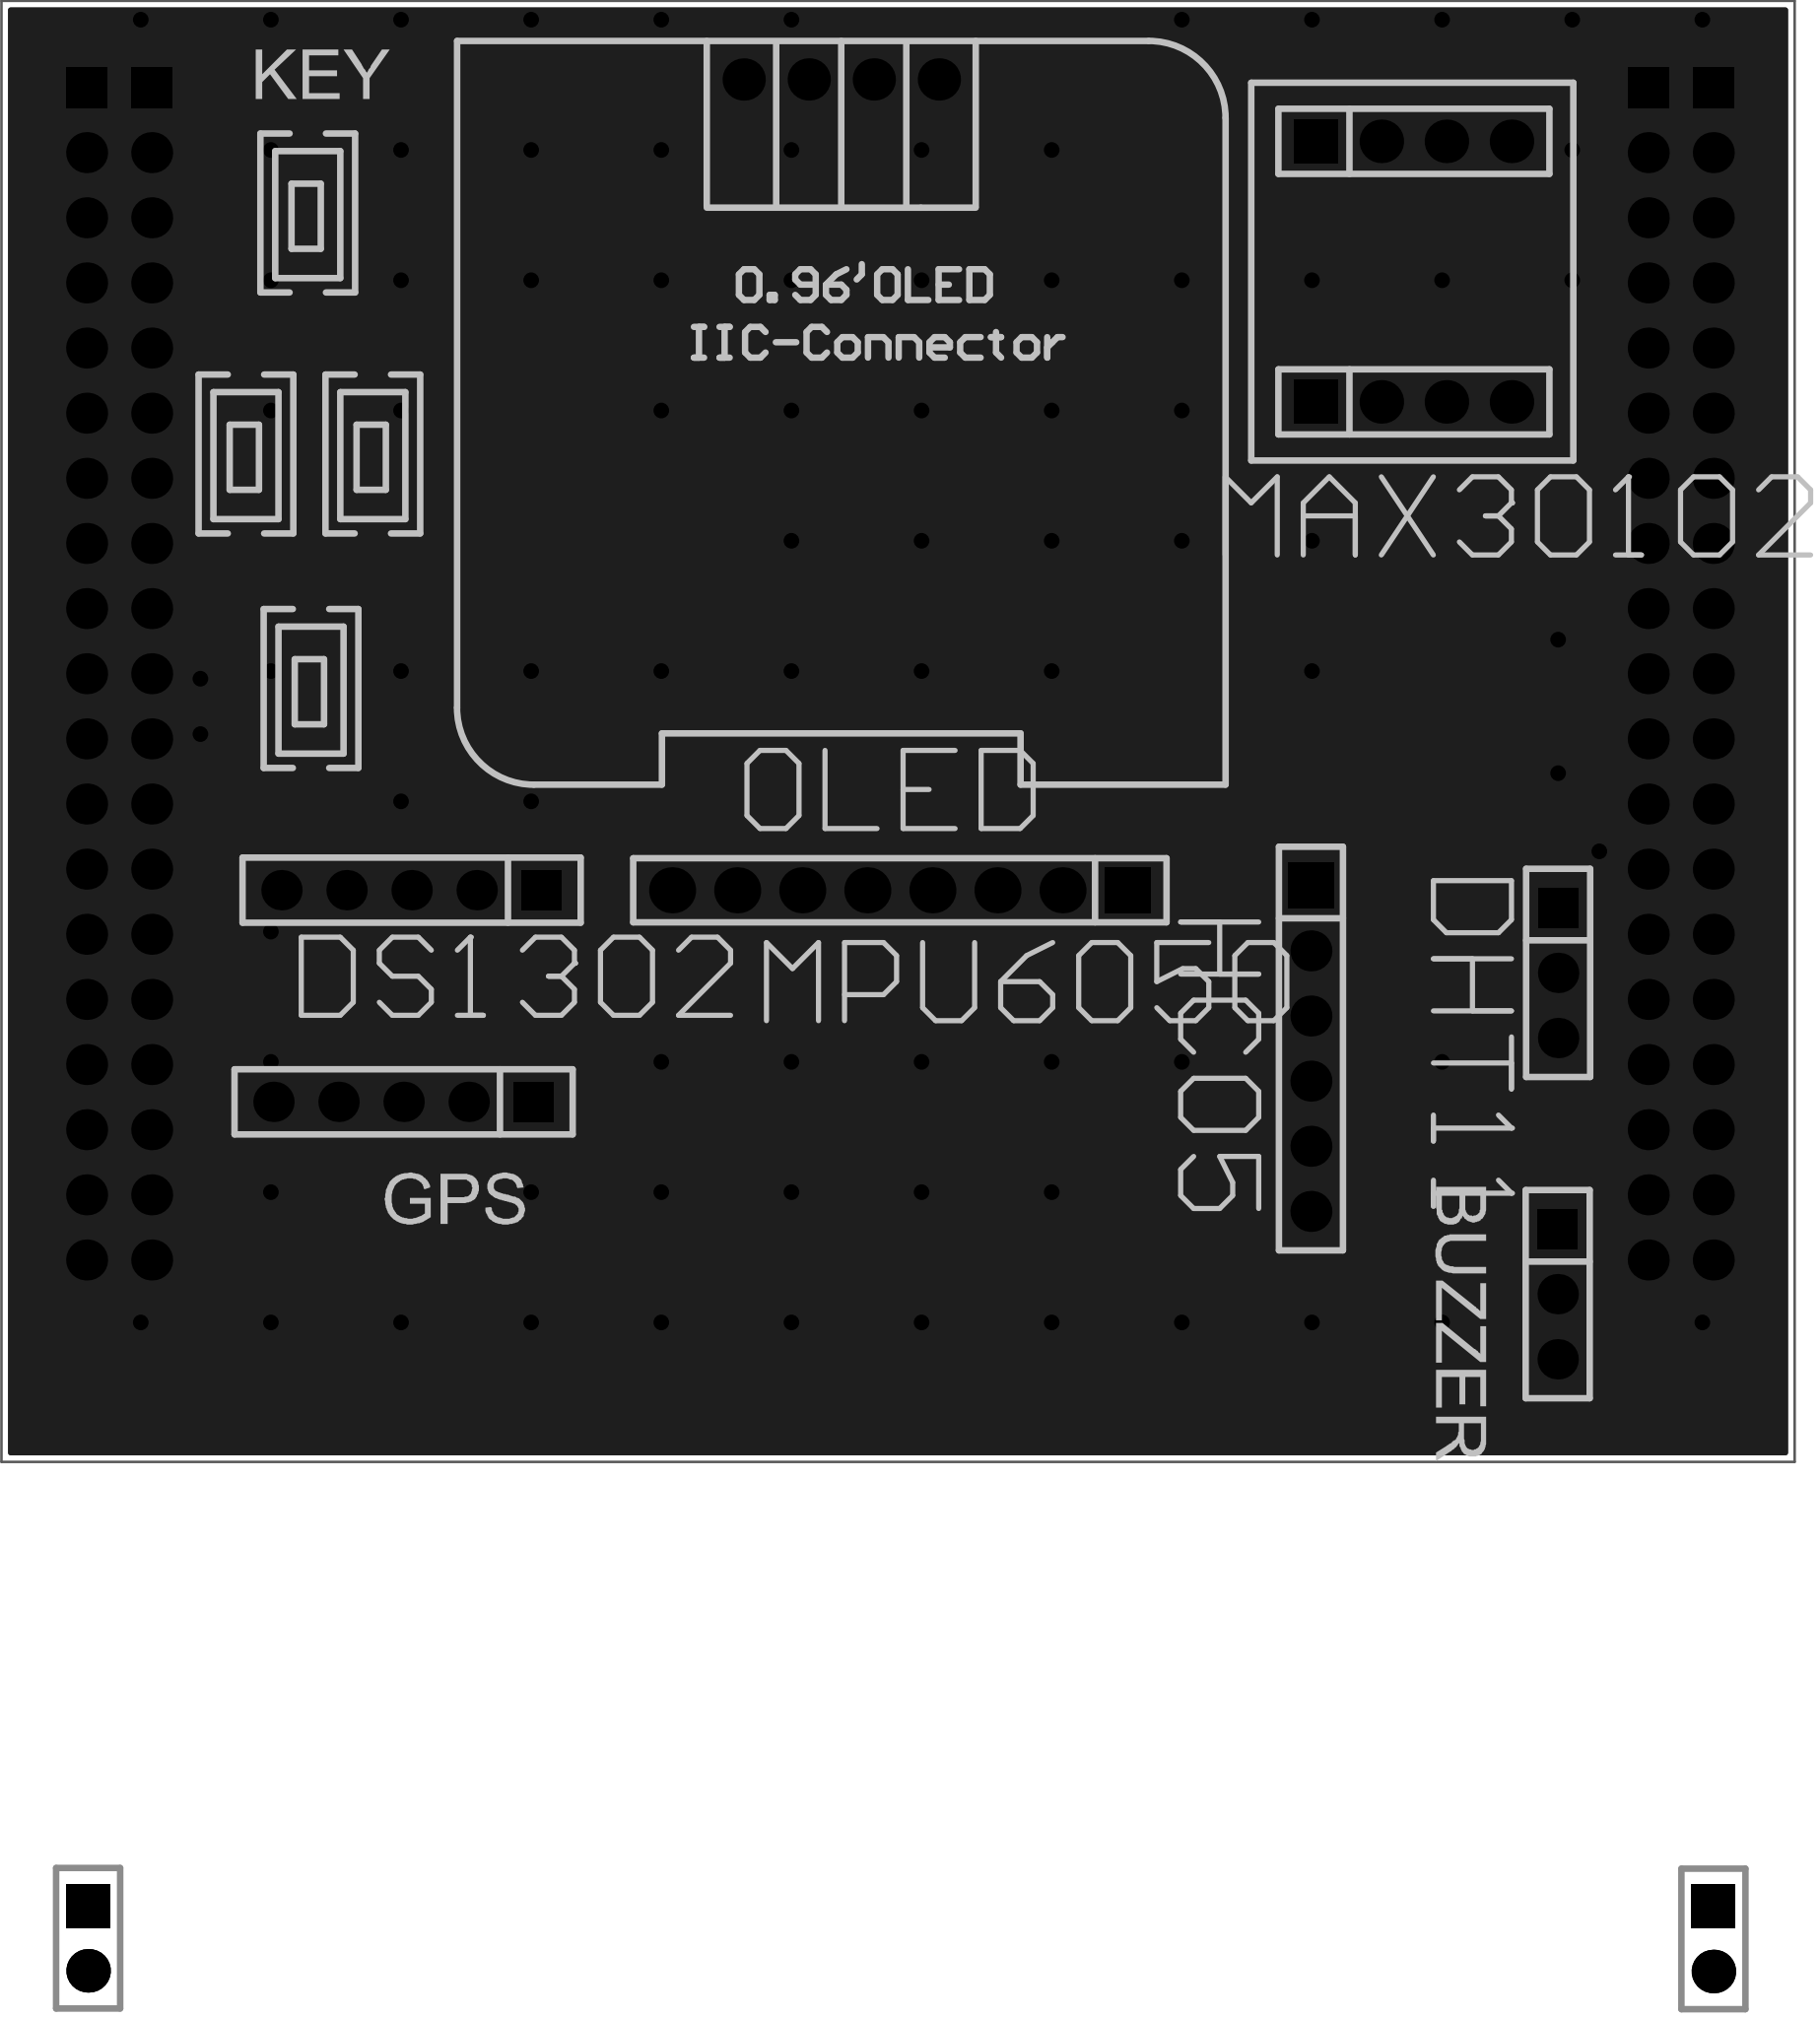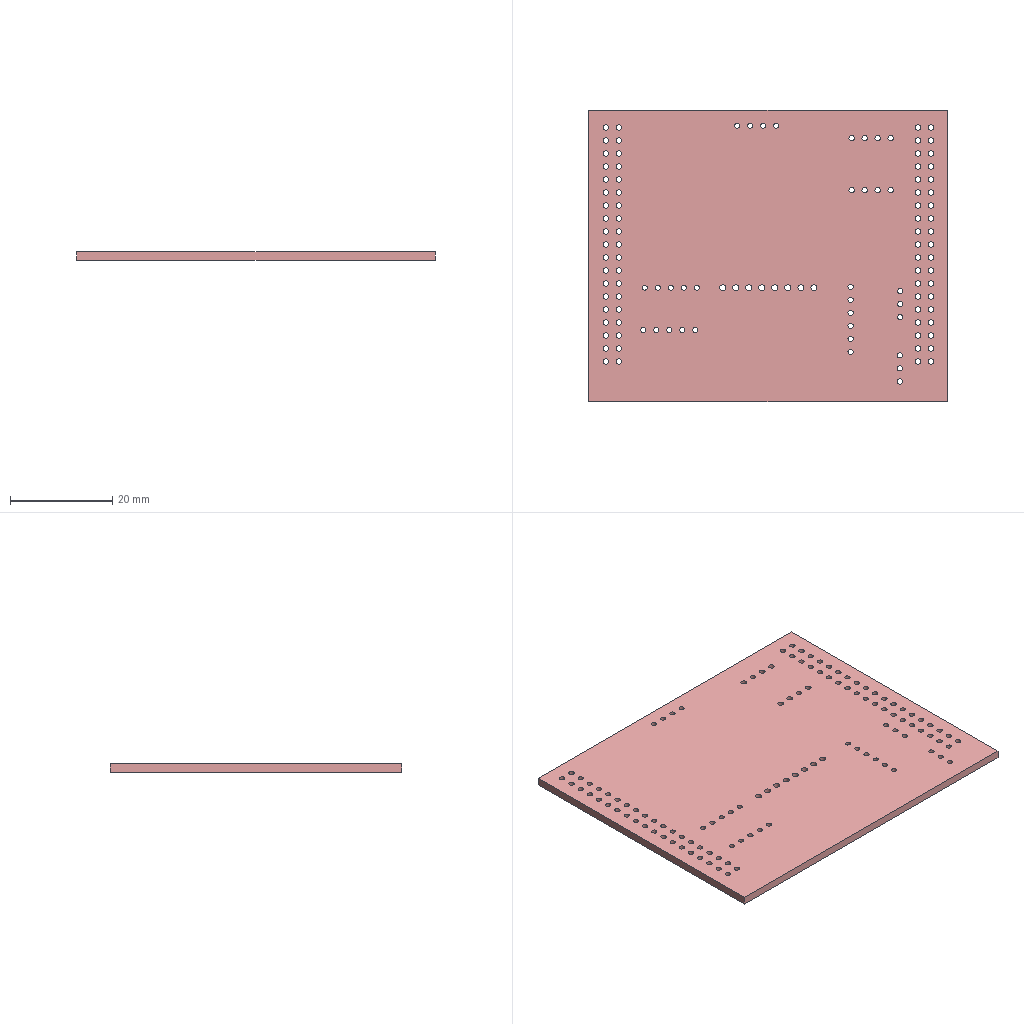Circuit board layout | Altium Designer | box 70 x 57 x 1.6 mm
Layer stack:
# Altium Designer layer stack of  (unit mm; dielectric type: 0 none, 1 core, 2 prepreg, 3 surface material)
index,name,kind,layer,copper_thickness_mm,dielectric_type,dielectric_thickness_mm,dielectric_material,dielectric_constant
0,Top Paste Mask Layer,other,,,,,,
1,Top Silkscreen Layer,other,,,,,,
2,Top Solder Mask Layer,dielectric,,,3,0.01,,3.3
3,Top Layer,copper,Top Layer,0.035,,,,
4,Dielectric1,dielectric,,,3,1.51,FR4,4.5
5,Bottom Layer,copper,Bottom Layer,0.035,,,,
6,Bottom Solder Mask Layer,dielectric,,,3,0.01,,3.3
7,Bottom Silkscreen Layer,other,,,,,,
8,Bottom Paste Mask Layer,other,,,,,,
# drill layer pairs: low layer,high layer
drill_pair,Top Layer,Bottom Layer
Part placement:
Designator,Comment,Layer,Footprint,Center-X(mm),Center-Y(mm),Rotation
H1,C2897382,BottomLayer,HDR-TH_19P-P2.54-V-F,102.62,128.845,270
H2,C2897382,BottomLayer,HDR-TH_19P-P2.54-V-F,105.16,128.845,270
H3,,TopLayer,HDR-TH_6P-P2.54-V-F,150.412,114.229,270
H4,,TopLayer,HDR-TH_8P-P2.54-V-F-1,134.366,120.401,180
H5,,TopLayer,HDR-TH_3P-P2.54-V-F,160.062,117.18,270
H6,,TopLayer,HDR-TH_3P-P2.54-V-F,160.045,104.653,270
H7,C2897382,BottomLayer,HDR-TH_19P-P2.54-V-F,163.58,128.845,270
H8,C2897382,BottomLayer,HDR-TH_19P-P2.54-V-F,166.12,128.845,270
H9,,TopLayer,HDR-TH_4P-P2.54-V-F,154.432,139.446,0
H10,,TopLayer,HDR-TH_4P-P2.54-V-F,154.432,149.606,0
H11,,TopLayer,HDR-TH_5P-P2.54-V-F,115.306,120.406,180
OLED1,,TopLayer,0.96OLED_4P,132.08,152.019,0
SW1,,TopLayer,Key_SMD_3.6x6.1x2.5,111.379,128.27,90
SW2,,TopLayer,Key_SMD_3.6x6.1x2.5,108.839,137.414,90
SW3,,TopLayer,Key_SMD_3.6x6.1x2.5,113.792,137.414,90
SW4,,TopLayer,Key_SMD_3.6x6.1x2.5,111.252,146.812,90
H12,,TopLayer,HDR-TH_5P-P2.54-V-F,114.993,112.151,180
H13,,BottomLayer,HDR-TH_2P-P2.54-V-F,102.678,79.537,270
H14,,BottomLayer,HDR-TH_2P-P2.54-V-F,166.124,79.51,270
Pad and via stacks:
# Altium Designer via and pad stacks of  (unit mm). Each distinct definition once, with the count of objects using it.
# via: kind,start_layer,end_layer,hole_mm,diameter_mm,mode(0 simple;1 top-mid-bottom;2 full stack),diameter_per_layer,count,example_net
# pad: kind,layer,hole_mm,hole_type(0 round;1 square;2 slot),plating,top_size,top_shape(1 round;2 rect;3 octagon;9 rounded rect),mid_size,bottom_size,mode,footprint,size_per_layer,count,example
pad,Multi-Layer,1.05,0,plated,1.6x1.6,1,1.6x1.6,1.6x1.6,0,HDR-TH_19P-P2.54-V-F,,72,H1.19
pad,Multi-Layer,1.05,0,plated,1.6x1.6,2,1.6x1.6,1.6x1.6,0,HDR-TH_19P-P2.54-V-F,,4,H1.1
pad,Multi-Layer,1.02,0,plated,1.6x1.6,1,1.6x1.6,1.6x1.6,0,HDR-TH_6P-P2.54-V-F,,5,H3.6
pad,Multi-Layer,1.02,0,plated,1.8x1.8,2,1.8x1.8,1.8x1.8,0,HDR-TH_6P-P2.54-V-F,,1,H3.1
pad,Multi-Layer,1.2,0,plated,1.8x1.8,2,1.8x1.8,1.8x1.8,0,HDR-TH_8P-P2.54-V-F-1,,1,H4.1
pad,Multi-Layer,1.2,0,plated,1.8x1.8,1,1.8x1.8,1.8x1.8,0,HDR-TH_8P-P2.54-V-F-1,,7,H4.2
pad,Multi-Layer,1.02,0,plated,1.575x1.575,1,1.575x1.575,1.575x1.575,0,HDR-TH_3P-P2.54-V-F,,4,H5.3
pad,Multi-Layer,1.02,0,plated,1.575x1.575,2,1.575x1.575,1.575x1.575,0,HDR-TH_3P-P2.54-V-F,,2,H5.1
pad,Multi-Layer,1.1,0,plated,1.7x1.7,2,1.7x1.7,1.7x1.7,0,HDR-TH_4P-P2.54-V-F,,2,H9.1
pad,Multi-Layer,1.1,0,plated,1.7x1.7,1,1.7x1.7,1.7x1.7,0,HDR-TH_4P-P2.54-V-F,,6,H9.2
pad,Multi-Layer,1.02,0,plated,1.575x1.575,1,1.575x1.575,1.575x1.575,0,HDR-TH_5P-P2.54-V-F,,8,H11.5
pad,Multi-Layer,1.02,0,plated,1.575x1.575,2,1.575x1.575,1.575x1.575,0,HDR-TH_5P-P2.54-V-F,,2,H11.1
pad,Multi-Layer,1,0,plated,1.65x1.65,1,1.65x1.65,1.65x1.65,0,0.96OLED_4P,,4,OLED1.4
pad,Multi-Layer,1,0,plated,1.7x1.7,2,1.7x1.7,1.7x1.7,0,HDR-TH_2P-P2.54-V-F,,2,H13.1
pad,Multi-Layer,1,0,plated,1.7x1.7,1,1.7x1.7,1.7x1.7,0,HDR-TH_2P-P2.54-V-F,,2,H13.2
pad,Top Layer,0,0,plated,1.501x1.001,2,1.501x1.001,1.501x1.001,0,Key_SMD_3.6x6.1x2.5,,8,SW1.2
via,Top Layer,Bottom Layer,0.3048,0.61,0,,83,CLK
Copper pours:
name,layer,net,type(0 solid;1 hatched;2 none)
Bottom Layer-GND,Bottom Layer,GND,0
Top Layer-GND,Top Layer,GND,0